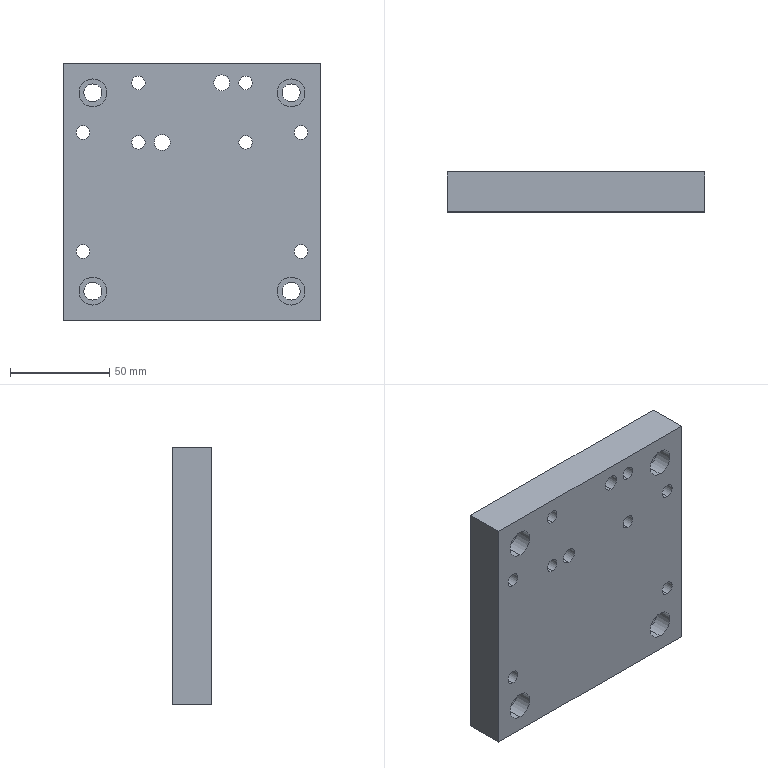Part | STEP file | OP10-137_base block (upper)-R | 1 solid | 64 faces | box 130 x 20 x 130 mm | volume 318432 mm3 | cylinder 48 | plane 16 | commonest cylinder face diameters 6.8 x8 7 x8 9 x8 11 x8 14 x8 8 x4